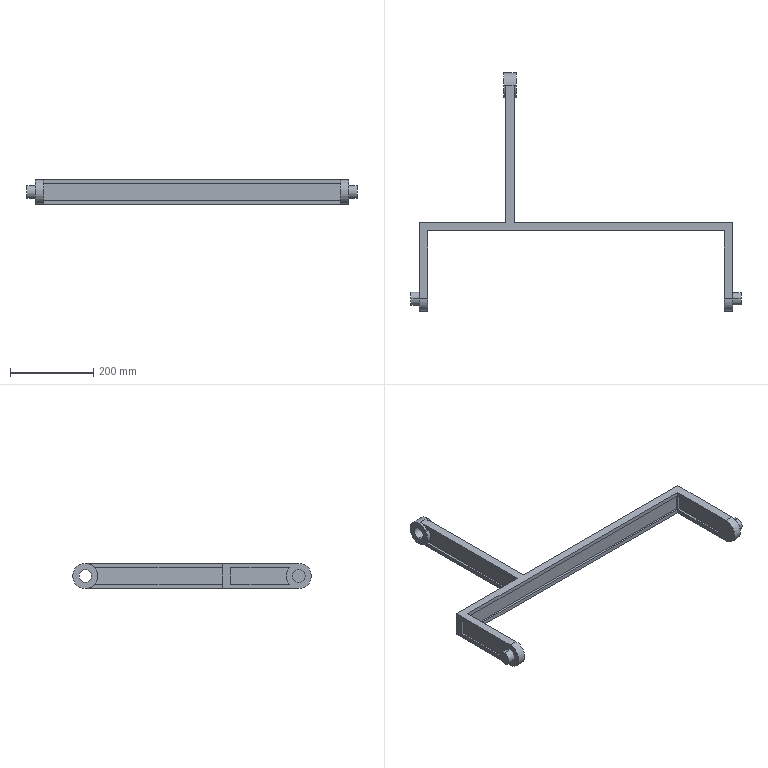Part | SolidWorks | features ICE 14, Extrusion 1 | 1 solid | 72 faces | box 794 x 573.5 x 60 mm | volume 1303043 mm3 | plane 57 | cylinder 15 | commonest cylinder face diameters 60 x9 30 x4 31 x2